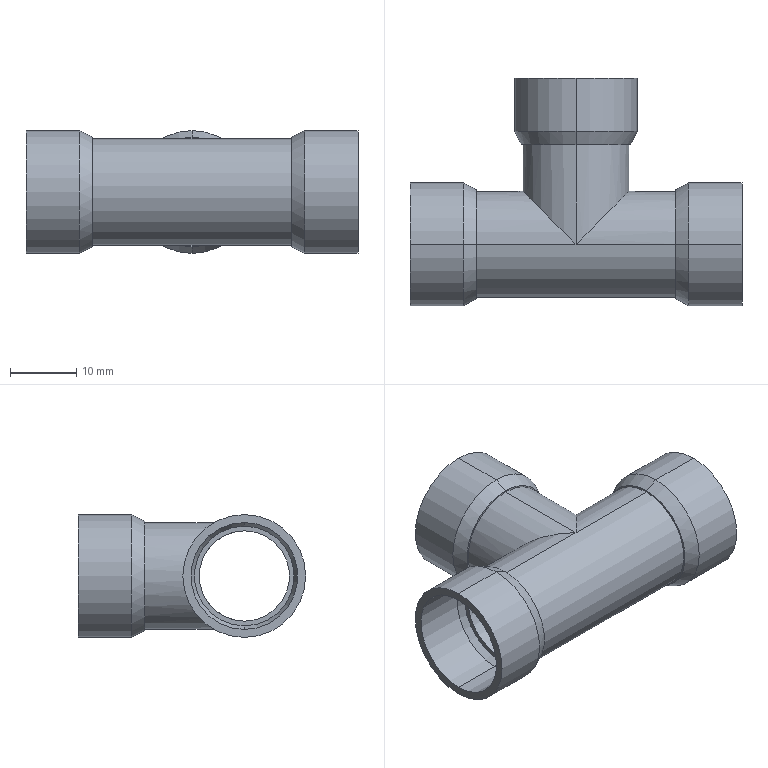Part | STEP file | tee copper tube | 1 solid | 43 faces | box 50 x 34.25 x 18.5 mm | volume 4026 mm3 | cylinder 22 | cone 12 | plane 9 | commonest cylinder face diameters 16.1 x6 18.5 x6 13.6 x5 16 x5